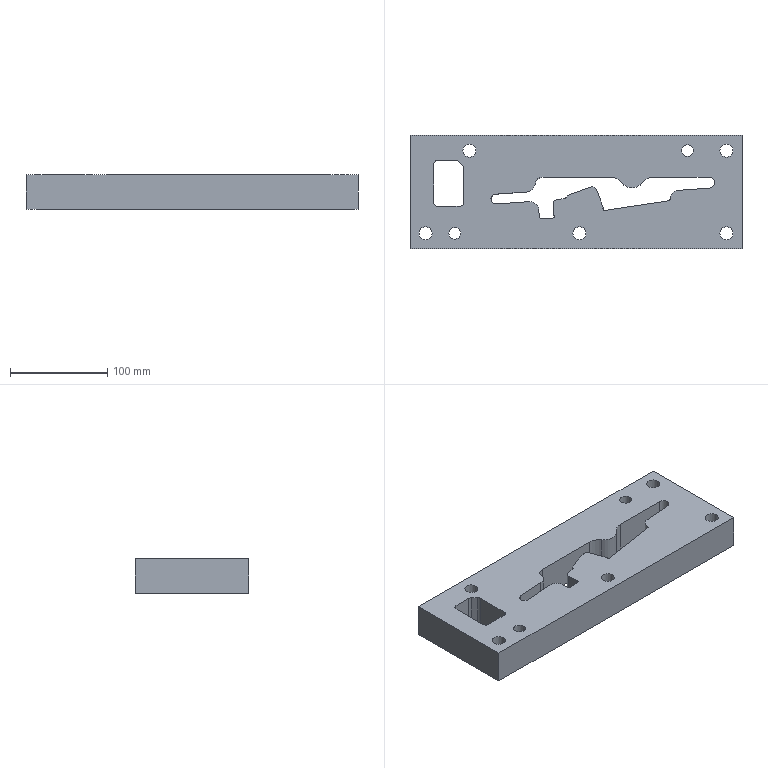Part | NX | features 7 2 | 1 solid | 108 faces | box 341 x 117 x 35 mm | volume 1112143 mm3 | cylinder 53 | plane 51 | cone 4 | commonest cylinder face diameters 10 x10 2 x6 20 x6 8 x5 13.5 x5 6.799 x4